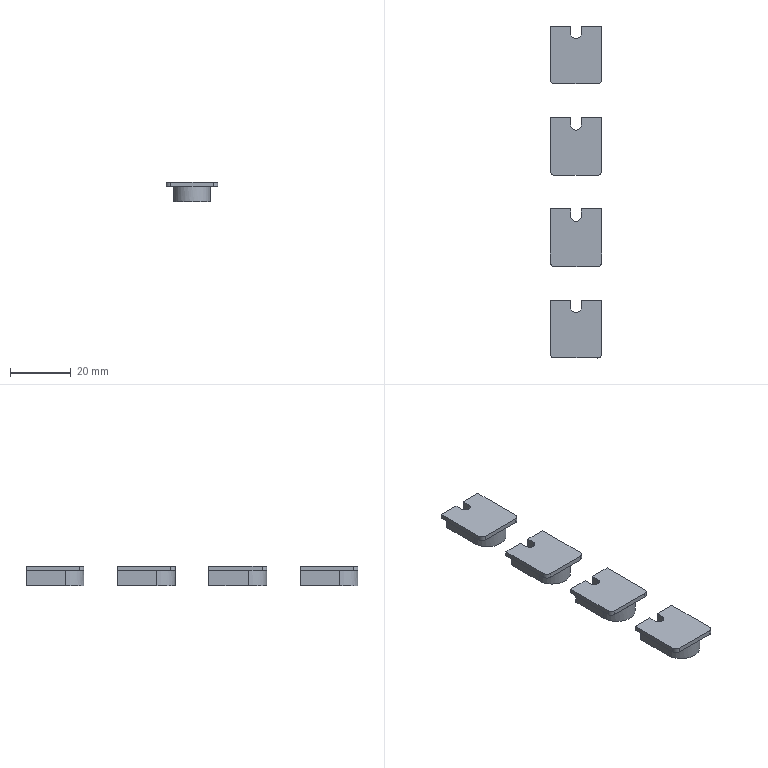Part | 4 solids | 96 faces | box 17.001 x 109 x 6.504 mm | volume 5564 mm3 | plane 72 | cylinder 20 | cone 4 | commonest cylinder face diameters 3 x8 3.4 x4 6.5 x4 12 x4